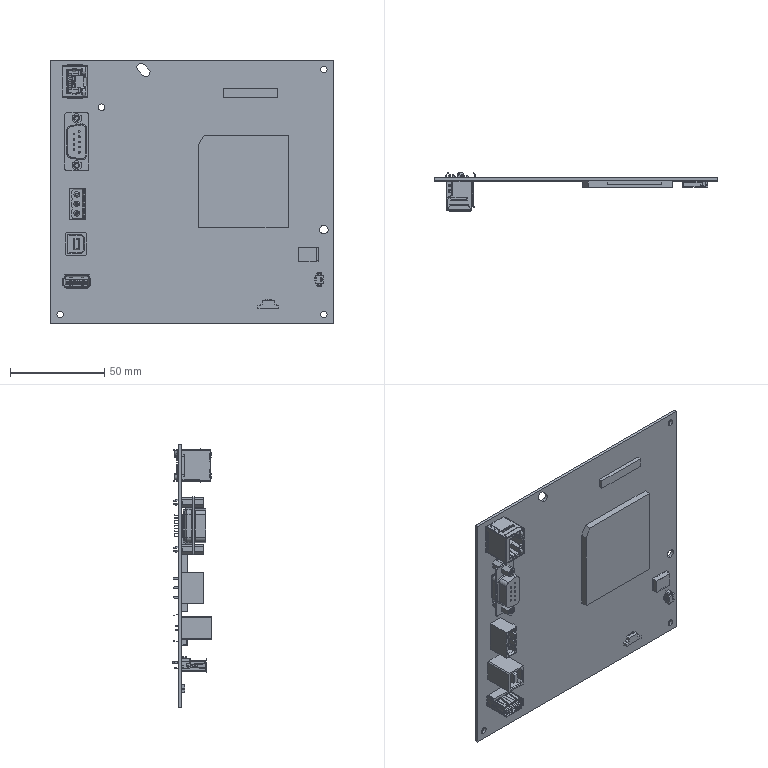Part | SolidWorks | 15 solids | 2449 faces | box 150 x 20.749 x 140 mm | volume 48945 mm3 | plane 1656 | cylinder 627 | spline 103 | torus 36 | cone 27 | commonest cylinder face diameters 0.5 x89 1 x74 0.4 x71 0.2 x48 0.6 x42 0.9 x40